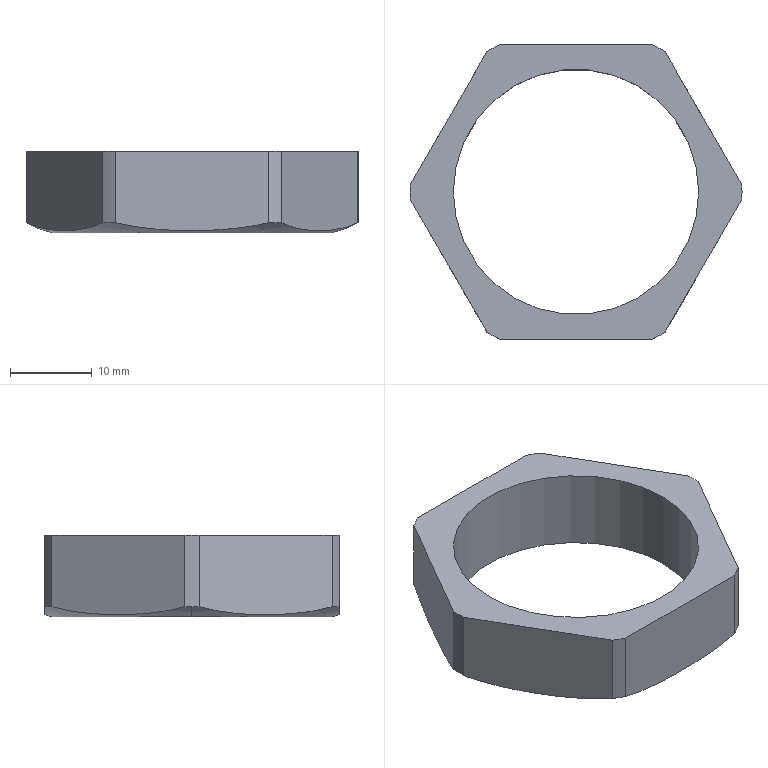Part | SolidWorks | features RefAxis 3, BaseBody 1 | 1 solid | 19 faces | box 40.6 x 36 x 10 mm | volume 4057 mm3 | cylinder 9 | plane 8 | spline 2 | commonest cylinder face diameters 40.6 x7 30 x2
STEP:
#1=CARTESIAN_POINT('',(35.75,19.99,0.));
#2=VERTEX_POINT('',#1);
#3=CARTESIAN_POINT('',(5.75,19.99,0.));
#4=VERTEX_POINT('',#3);
#5=CARTESIAN_POINT('',(20.75,19.99,0.));
#6=DIRECTION('',(0.,0.,-1.));
#7=DIRECTION('',(-1.,0.,0.));
#8=AXIS2_PLACEMENT_3D('',#5,#6,#7);
#9=CIRCLE('',#8,15.);
#10=EDGE_CURVE('',#2,#4,#9,.T.);
#11=ORIENTED_EDGE('',*,*,#10,.F.);
#12=CARTESIAN_POINT('',(35.75,19.99,-10.));
#13=VERTEX_POINT('',#12);
#14=CARTESIAN_POINT('',(35.75,19.99,0.));
#15=DIRECTION('',(0.,0.,-1.));
#16=VECTOR('',#15,1000.);
#17=LINE('',#14,#16);
#18=EDGE_CURVE('',#2,#13,#17,.T.);
#19=ORIENTED_EDGE('',*,*,#18,.T.);
#20=CARTESIAN_POINT('',(5.75,19.99,-10.));
#21=VERTEX_POINT('',#20);
#22=CARTESIAN_POINT('',(20.75,19.99,-10.));
#23=DIRECTION('',(0.,0.,1.));
#24=DIRECTION('',(-1.,0.,0.));
#25=AXIS2_PLACEMENT_3D('',#22,#23,#24);
#26=CIRCLE('',#25,15.);
#27=EDGE_CURVE('',#21,#13,#26,.T.);
#28=ORIENTED_EDGE('',*,*,#27,.F.);
#29=CARTESIAN_POINT('',(5.75,19.99,0.));
#30=DIRECTION('',(0.,0.,-1.));
#31=VECTOR('',#30,1000.);
#32=LINE('',#29,#31);
#33=EDGE_CURVE('',#4,#21,#32,.T.);
#34=ORIENTED_EDGE('',*,*,#33,.F.);
#35=EDGE_LOOP('',(#11,#19,#28,#34));
#36=FACE_OUTER_BOUND('',#35,.T.);
#37=CARTESIAN_POINT('',(20.75,19.99,0.));
#38=DIRECTION('',(0.,0.,-1.));
#39=DIRECTION('',(-1.,0.,0.));
#40=AXIS2_PLACEMENT_3D('',#37,#38,#39);
#41=CYLINDRICAL_SURFACE('',#40,15.);
#42=ADVANCED_FACE('',(#36),#41,.F.);
#43=CARTESIAN_POINT('',(41.031,19.118,-8.75));
#44=VERTEX_POINT('',#43);
#45=CARTESIAN_POINT('',(41.05,19.99,-8.75));
#46=VERTEX_POINT('',#45);
#47=CARTESIAN_POINT('',(20.75,19.99,-8.75));
#48=DIRECTION('',(0.,0.,1.));
#49=DIRECTION('',(1.,0.,0.));
#50=AXIS2_PLACEMENT_3D('',#47,#48,#49);
#51=CIRCLE('',#50,20.3);
#52=EDGE_CURVE('',#44,#46,#51,.T.);
#53=ORIENTED_EDGE('',*,*,#52,.T.);
#54=CARTESIAN_POINT('',(41.05,19.99,0.));
#55=VERTEX_POINT('',#54);
#56=CARTESIAN_POINT('',(41.05,19.99,-11.417));
#57=DIRECTION('',(0.,0.,1.));
#58=VECTOR('',#57,1000.);
#59=LINE('',#56,#58);
#60=EDGE_CURVE('',#46,#55,#59,.T.);
#61=ORIENTED_EDGE('',*,*,#60,.T.);
#62=CARTESIAN_POINT('',(41.031,19.118,0.));
#63=VERTEX_POINT('',#62);
#64=CARTESIAN_POINT('',(20.75,19.99,0.));
#65=DIRECTION('',(0.,0.,-1.));
#66=DIRECTION('',(1.,0.,0.));
#67=AXIS2_PLACEMENT_3D('',#64,#65,#66);
#68=CIRCLE('',#67,20.3);
#69=EDGE_CURVE('',#55,#63,#68,.T.);
#70=ORIENTED_EDGE('',*,*,#69,.T.);
#71=CARTESIAN_POINT('',(41.031,19.118,0.));
#72=DIRECTION('',(0.,0.,-1.));
#73=VECTOR('',#72,1000.);
#74=LINE('',#71,#73);
#75=EDGE_CURVE('',#63,#44,#74,.T.);
#76=ORIENTED_EDGE('',*,*,#75,.T.);
#77=EDGE_LOOP('',(#53,#61,#70,#76));
#78=FACE_OUTER_BOUND('',#77,.T.);
#79=CARTESIAN_POINT('',(20.75,19.99,-11.417));
#80=DIRECTION('',(0.,0.,1.));
#81=DIRECTION('',(1.,0.,0.));
#82=AXIS2_PLACEMENT_3D('',#79,#80,#81);
#83=CYLINDRICAL_SURFACE('',#82,20.3);
#84=ADVANCED_FACE('',(#78),#83,.T.);
#85=ORIENTED_EDGE('',*,*,#18,.F.);
#86=CARTESIAN_POINT('',(20.75,19.99,0.));
#87=DIRECTION('',(0.,0.,-1.));
#88=DIRECTION('',(-1.,0.,0.));
#89=AXIS2_PLACEMENT_3D('',#86,#87,#88);
#90=CIRCLE('',#89,15.);
#91=EDGE_CURVE('',#4,#2,#90,.T.);
#92=ORIENTED_EDGE('',*,*,#91,.F.);
#93=ORIENTED_EDGE('',*,*,#33,.T.);
#94=CARTESIAN_POINT('',(20.75,19.99,-10.));
#95=DIRECTION('',(0.,0.,1.));
#96=DIRECTION('',(-1.,0.,0.));
#97=AXIS2_PLACEMENT_3D('',#94,#95,#96);
#98=CIRCLE('',#97,15.);
#99=EDGE_CURVE('',#13,#21,#98,.T.);
#100=ORIENTED_EDGE('',*,*,#99,.F.);
#101=EDGE_LOOP('',(#85,#92,#93,#100));
#102=FACE_OUTER_BOUND('',#101,.T.);
#103=CARTESIAN_POINT('',(20.75,19.99,0.));
#104=DIRECTION('',(0.,0.,-1.));
#105=DIRECTION('',(-1.,0.,0.));
#106=AXIS2_PLACEMENT_3D('',#103,#104,#105);
#107=CYLINDRICAL_SURFACE('',#106,15.);
#108=ADVANCED_FACE('',(#102),#107,.F.);
#109=ORIENTED_EDGE('',*,*,#91,.T.);
#110=ORIENTED_EDGE('',*,*,#10,.T.);
#111=EDGE_LOOP('',(#109,#110));
#112=FACE_BOUND('',#111,.T.);
#113=CARTESIAN_POINT('',(41.031,20.862,0.));
#114=VERTEX_POINT('',#113);
#115=CARTESIAN_POINT('',(20.75,19.99,0.));
#116=DIRECTION('',(0.,0.,-1.));
#117=DIRECTION('',(1.,0.,0.));
#118=AXIS2_PLACEMENT_3D('',#115,#116,#117);
#119=CIRCLE('',#118,20.3);
#120=EDGE_CURVE('',#114,#55,#119,.T.);
#121=ORIENTED_EDGE('',*,*,#120,.F.);
#122=CARTESIAN_POINT('',(31.646,37.118,0.));
#123=VERTEX_POINT('',#122);
#124=CARTESIAN_POINT('',(41.031,20.862,0.));
#125=DIRECTION('',(-0.5,0.866,0.));
#126=VECTOR('',#125,1000.);
#127=LINE('',#124,#126);
#128=EDGE_CURVE('',#114,#123,#127,.T.);
#129=ORIENTED_EDGE('',*,*,#128,.T.);
#130=CARTESIAN_POINT('',(30.136,37.99,0.));
#131=VERTEX_POINT('',#130);
#132=CARTESIAN_POINT('',(20.75,19.99,0.));
#133=DIRECTION('',(0.,0.,1.));
#134=DIRECTION('',(1.,0.,0.));
#135=AXIS2_PLACEMENT_3D('',#132,#133,#134);
#136=CIRCLE('',#135,20.3);
#137=EDGE_CURVE('',#123,#131,#136,.T.);
#138=ORIENTED_EDGE('',*,*,#137,.T.);
#139=CARTESIAN_POINT('',(11.364,37.99,0.));
#140=VERTEX_POINT('',#139);
#141=CARTESIAN_POINT('',(41.535,37.99,0.));
#142=DIRECTION('',(-1.,0.,0.));
#143=VECTOR('',#142,1000.);
#144=LINE('',#141,#143);
#145=EDGE_CURVE('',#131,#140,#144,.T.);
#146=ORIENTED_EDGE('',*,*,#145,.T.);
#147=CARTESIAN_POINT('',(9.854,37.118,0.));
#148=VERTEX_POINT('',#147);
#149=CARTESIAN_POINT('',(20.75,19.99,0.));
#150=DIRECTION('',(0.,0.,1.));
#151=DIRECTION('',(1.,0.,0.));
#152=AXIS2_PLACEMENT_3D('',#149,#150,#151);
#153=CIRCLE('',#152,20.3);
#154=EDGE_CURVE('',#140,#148,#153,.T.);
#155=ORIENTED_EDGE('',*,*,#154,.T.);
#156=CARTESIAN_POINT('',(0.4687,20.862,0.));
#157=VERTEX_POINT('',#156);
#158=CARTESIAN_POINT('',(9.854,37.118,0.));
#159=DIRECTION('',(-0.5,-0.866,0.));
#160=VECTOR('',#159,1000.);
#161=LINE('',#158,#160);
#162=EDGE_CURVE('',#148,#157,#161,.T.);
#163=ORIENTED_EDGE('',*,*,#162,.T.);
#164=CARTESIAN_POINT('',(0.4687,19.118,0.));
#165=VERTEX_POINT('',#164);
#166=CARTESIAN_POINT('',(20.75,19.99,0.));
#167=DIRECTION('',(0.,0.,1.));
#168=DIRECTION('',(1.,0.,0.));
#169=AXIS2_PLACEMENT_3D('',#166,#167,#168);
#170=CIRCLE('',#169,20.3);
#171=EDGE_CURVE('',#157,#165,#170,.T.);
#172=ORIENTED_EDGE('',*,*,#171,.T.);
#173=CARTESIAN_POINT('',(9.854,2.862,0.));
#174=VERTEX_POINT('',#173);
#175=CARTESIAN_POINT('',(0.4687,19.118,0.));
#176=DIRECTION('',(0.5,-0.866,0.));
#177=VECTOR('',#176,1000.);
#178=LINE('',#175,#177);
#179=EDGE_CURVE('',#165,#174,#178,.T.);
#180=ORIENTED_EDGE('',*,*,#179,.T.);
#181=CARTESIAN_POINT('',(11.364,1.99,0.));
#182=VERTEX_POINT('',#181);
#183=CARTESIAN_POINT('',(20.75,19.99,0.));
#184=DIRECTION('',(0.,0.,1.));
#185=DIRECTION('',(1.,0.,0.));
#186=AXIS2_PLACEMENT_3D('',#183,#184,#185);
#187=CIRCLE('',#186,20.3);
#188=EDGE_CURVE('',#174,#182,#187,.T.);
#189=ORIENTED_EDGE('',*,*,#188,.T.);
#190=CARTESIAN_POINT('',(30.136,1.99,0.));
#191=VERTEX_POINT('',#190);
#192=CARTESIAN_POINT('',(41.535,1.99,0.));
#193=DIRECTION('',(1.,0.,0.));
#194=VECTOR('',#193,1000.);
#195=LINE('',#192,#194);
#196=EDGE_CURVE('',#182,#191,#195,.T.);
#197=ORIENTED_EDGE('',*,*,#196,.T.);
#198=CARTESIAN_POINT('',(31.646,2.862,0.));
#199=VERTEX_POINT('',#198);
#200=CARTESIAN_POINT('',(20.75,19.99,0.));
#201=DIRECTION('',(0.,0.,1.));
#202=DIRECTION('',(1.,0.,0.));
#203=AXIS2_PLACEMENT_3D('',#200,#201,#202);
#204=CIRCLE('',#203,20.3);
#205=EDGE_CURVE('',#191,#199,#204,.T.);
#206=ORIENTED_EDGE('',*,*,#205,.T.);
#207=CARTESIAN_POINT('',(31.646,2.862,0.));
#208=DIRECTION('',(0.5,0.866,0.));
#209=VECTOR('',#208,1000.);
#210=LINE('',#207,#209);
#211=EDGE_CURVE('',#199,#63,#210,.T.);
#212=ORIENTED_EDGE('',*,*,#211,.T.);
#213=ORIENTED_EDGE('',*,*,#69,.F.);
#214=EDGE_LOOP('',(#121,#129,#138,#146,#155,#163,#172,#180,#189,#197,#206,#212,#213));
#215=FACE_OUTER_BOUND('',#214,.T.);
#216=CARTESIAN_POINT('',(41.535,19.99,0.));
#217=DIRECTION('',(0.,0.,1.));
#218=DIRECTION('',(1.,0.,0.));
#219=AXIS2_PLACEMENT_3D('',#216,#217,#218);
#220=PLANE('',#219);
#221=ADVANCED_FACE('',(#112,#215),#220,.T.);
#222=ORIENTED_EDGE('',*,*,#27,.T.);
#223=ORIENTED_EDGE('',*,*,#99,.T.);
#224=EDGE_LOOP('',(#222,#223));
#225=FACE_BOUND('',#224,.T.);
#226=CARTESIAN_POINT('',(37.75,19.99,-10.));
#227=VERTEX_POINT('',#226);
#228=CARTESIAN_POINT('',(3.75,19.99,-10.));
#229=VERTEX_POINT('',#228);
#230=CARTESIAN_POINT('',(37.75,19.99,-10.));
#231=CARTESIAN_POINT('',(37.75,53.99,-10.));
#232=CARTESIAN_POINT('',(3.75,53.99,-10.));
#233=CARTESIAN_POINT('',(3.75,19.99,-10.));
#234=(BOUNDED_CURVE()B_SPLINE_CURVE(3,(#230,#231,#232,#233),.UNSPECIFIED.,.F.,.F.)B_SPLINE_CURVE_WITH_KNOTS((4,4),(0.,0.05314),.UNSPECIFIED.)CURVE()GEOMETRIC_REPRESENTATION_ITEM()RATIONAL_B_SPLINE_CURVE((1.,0.3333,0.3333,1.))REPRESENTATION_ITEM(''));
#235=EDGE_CURVE('',#227,#229,#234,.T.);
#236=ORIENTED_EDGE('',*,*,#235,.F.);
#237=CARTESIAN_POINT('',(3.75,19.99,-10.));
#238=CARTESIAN_POINT('',(3.75,-14.01,-10.));
#239=CARTESIAN_POINT('',(37.75,-14.01,-10.));
#240=CARTESIAN_POINT('',(37.75,19.99,-10.));
#241=(BOUNDED_CURVE()B_SPLINE_CURVE(3,(#237,#238,#239,#240),.UNSPECIFIED.,.F.,.F.)B_SPLINE_CURVE_WITH_KNOTS((4,4),(0.,0.05314),.UNSPECIFIED.)CURVE()GEOMETRIC_REPRESENTATION_ITEM()RATIONAL_B_SPLINE_CURVE((1.,0.3333,0.3333,1.))REPRESENTATION_ITEM(''));
#242=EDGE_CURVE('',#229,#227,#241,.T.);
#243=ORIENTED_EDGE('',*,*,#242,.F.);
#244=EDGE_LOOP('',(#236,#243));
#245=FACE_OUTER_BOUND('',#244,.T.);
#246=CARTESIAN_POINT('',(41.535,19.99,-10.));
#247=DIRECTION('',(0.,0.,1.));
#248=DIRECTION('',(1.,0.,0.));
#249=AXIS2_PLACEMENT_3D('',#246,#247,#248);
#250=PLANE('',#249);
#251=ADVANCED_FACE('',(#225,#245),#250,.F.);
#252=CARTESIAN_POINT('',(31.646,2.862,-8.75));
#253=VERTEX_POINT('',#252);
#254=CARTESIAN_POINT('',(31.646,2.862,0.));
#255=DIRECTION('',(0.,0.,1.));
#256=VECTOR('',#255,1000.);
#257=LINE('',#254,#256);
#258=EDGE_CURVE('',#253,#199,#257,.T.);
#259=ORIENTED_EDGE('',*,*,#258,.F.);
#260=CARTESIAN_POINT('',(41.031,19.118,-8.75));
#261=CARTESIAN_POINT('',(40.646,18.451,-8.942));
#262=CARTESIAN_POINT('',(40.258,17.778,-9.096));
#263=CARTESIAN_POINT('',(39.475,16.424,-9.345));
#264=CARTESIAN_POINT('',(39.081,15.74,-9.441));
#265=CARTESIAN_POINT('',(37.899,13.694,-9.662));
#266=CARTESIAN_POINT('',(37.114,12.333,-9.722));
#267=CARTESIAN_POINT('',(35.545,9.616,-9.721));
#268=CARTESIAN_POINT('',(34.762,8.259,-9.659));
#269=CARTESIAN_POINT('',(33.2,5.554,-9.367));
#270=CARTESIAN_POINT('',(32.421,4.205,-9.137));
#271=CARTESIAN_POINT('',(31.646,2.862,-8.75));
#272=B_SPLINE_CURVE_WITH_KNOTS('',3,(#260,#261,#262,#263,#264,#265,#266,#267,#268,#269,#270,#271),.UNSPECIFIED.,.F.,.F.,(4,2,2,2,2,4),(0.,0.002376,0.004751,0.009503,0.01425,0.01901),.UNSPECIFIED.);
#273=EDGE_CURVE('',#44,#253,#272,.T.);
#274=ORIENTED_EDGE('',*,*,#273,.F.);
#275=ORIENTED_EDGE('',*,*,#75,.F.);
#276=ORIENTED_EDGE('',*,*,#211,.F.);
#277=EDGE_LOOP('',(#259,#274,#275,#276));
#278=FACE_OUTER_BOUND('',#277,.T.);
#279=CARTESIAN_POINT('',(31.142,1.99,0.));
#280=DIRECTION('',(-0.866,0.5,0.));
#281=DIRECTION('',(-0.5,-0.866,0.));
#282=AXIS2_PLACEMENT_3D('',#279,#280,#281);
#283=PLANE('',#282);
#284=ADVANCED_FACE('',(#278),#283,.F.);
#285=ORIENTED_EDGE('',*,*,#205,.F.);
#286=CARTESIAN_POINT('',(30.136,1.99,-8.75));
#287=VERTEX_POINT('',#286);
#288=CARTESIAN_POINT('',(30.136,1.99,-11.417));
#289=DIRECTION('',(0.,0.,-1.));
#290=VECTOR('',#289,1000.);
#291=LINE('',#288,#290);
#292=EDGE_CURVE('',#191,#287,#291,.T.);
#293=ORIENTED_EDGE('',*,*,#292,.T.);
#294=CARTESIAN_POINT('',(20.75,19.99,-8.75));
#295=DIRECTION('',(0.,0.,1.));
#296=DIRECTION('',(1.,0.,0.));
#297=AXIS2_PLACEMENT_3D('',#294,#295,#296);
#298=CIRCLE('',#297,20.3);
#299=EDGE_CURVE('',#287,#253,#298,.T.);
#300=ORIENTED_EDGE('',*,*,#299,.T.);
#301=ORIENTED_EDGE('',*,*,#258,.T.);
#302=EDGE_LOOP('',(#285,#293,#300,#301));
#303=FACE_OUTER_BOUND('',#302,.T.);
#304=CARTESIAN_POINT('',(20.75,19.99,-11.417));
#305=DIRECTION('',(0.,0.,1.));
#306=DIRECTION('',(1.,0.,0.));
#307=AXIS2_PLACEMENT_3D('',#304,#305,#306);
#308=CYLINDRICAL_SURFACE('',#307,20.3);
#309=ADVANCED_FACE('',(#303),#308,.T.);
#310=CARTESIAN_POINT('',(11.364,1.99,-8.75));
#311=VERTEX_POINT('',#310);
#312=CARTESIAN_POINT('',(11.364,1.99,0.));
#313=DIRECTION('',(0.,0.,1.));
#314=VECTOR('',#313,1000.);
#315=LINE('',#312,#314);
#316=EDGE_CURVE('',#311,#182,#315,.T.);
#317=ORIENTED_EDGE('',*,*,#316,.F.);
#318=CARTESIAN_POINT('',(30.136,1.99,-8.75));
#319=CARTESIAN_POINT('',(28.596,1.99,-9.134));
#320=CARTESIAN_POINT('',(27.029,1.99,-9.367));
#321=CARTESIAN_POINT('',(23.875,1.99,-9.662));
#322=CARTESIAN_POINT('',(22.302,1.99,-9.722));
#323=CARTESIAN_POINT('',(19.162,1.99,-9.721));
#324=CARTESIAN_POINT('',(17.596,1.99,-9.659));
#325=CARTESIAN_POINT('',(14.472,1.99,-9.367));
#326=CARTESIAN_POINT('',(12.914,1.99,-9.136));
#327=CARTESIAN_POINT('',(11.364,1.99,-8.75));
#328=B_SPLINE_CURVE_WITH_KNOTS('',3,(#318,#319,#320,#321,#322,#323,#324,#325,#326,#327),.UNSPECIFIED.,.F.,.F.,(4,2,2,2,4),(0.,0.004746,0.009492,0.01424,0.01898),.UNSPECIFIED.);
#329=EDGE_CURVE('',#287,#311,#328,.T.);
#330=ORIENTED_EDGE('',*,*,#329,.F.);
#331=ORIENTED_EDGE('',*,*,#292,.F.);
#332=ORIENTED_EDGE('',*,*,#196,.F.);
#333=EDGE_LOOP('',(#317,#330,#331,#332));
#334=FACE_OUTER_BOUND('',#333,.T.);
#335=CARTESIAN_POINT('',(10.358,1.99,0.));
#336=DIRECTION('',(0.,1.,0.));
#337=DIRECTION('',(-1.,0.,0.));
#338=AXIS2_PLACEMENT_3D('',#335,#336,#337);
#339=PLANE('',#338);
#340=ADVANCED_FACE('',(#334),#339,.F.);
#341=ORIENTED_EDGE('',*,*,#188,.F.);
#342=CARTESIAN_POINT('',(9.854,2.862,-8.75));
#343=VERTEX_POINT('',#342);
#344=CARTESIAN_POINT('',(9.854,2.862,-11.417));
#345=DIRECTION('',(0.,0.,-1.));
#346=VECTOR('',#345,1000.);
#347=LINE('',#344,#346);
#348=EDGE_CURVE('',#174,#343,#347,.T.);
#349=ORIENTED_EDGE('',*,*,#348,.T.);
#350=CARTESIAN_POINT('',(20.75,19.99,-8.75));
#351=DIRECTION('',(0.,0.,1.));
#352=DIRECTION('',(1.,0.,0.));
#353=AXIS2_PLACEMENT_3D('',#350,#351,#352);
#354=CIRCLE('',#353,20.3);
#355=EDGE_CURVE('',#343,#311,#354,.T.);
#356=ORIENTED_EDGE('',*,*,#355,.T.);
#357=ORIENTED_EDGE('',*,*,#316,.T.);
#358=EDGE_LOOP('',(#341,#349,#356,#357));
#359=FACE_OUTER_BOUND('',#358,.T.);
#360=CARTESIAN_POINT('',(20.75,19.99,-11.417));
#361=DIRECTION('',(0.,0.,1.));
#362=DIRECTION('',(1.,0.,0.));
#363=AXIS2_PLACEMENT_3D('',#360,#361,#362);
#364=CYLINDRICAL_SURFACE('',#363,20.3);
#365=ADVANCED_FACE('',(#359),#364,.T.);
#366=CARTESIAN_POINT('',(0.4687,19.118,-8.75));
#367=VERTEX_POINT('',#366);
#368=CARTESIAN_POINT('',(0.4687,19.118,0.));
#369=DIRECTION('',(0.,0.,1.));
#370=VECTOR('',#369,1000.);
#371=LINE('',#368,#370);
#372=EDGE_CURVE('',#367,#165,#371,.T.);
#373=ORIENTED_EDGE('',*,*,#372,.F.);
#374=CARTESIAN_POINT('',(9.854,2.862,-8.75));
#375=CARTESIAN_POINT('',(9.084,4.195,-9.134));
#376=CARTESIAN_POINT('',(8.301,5.552,-9.367));
#377=CARTESIAN_POINT('',(6.724,8.284,-9.662));
#378=CARTESIAN_POINT('',(5.937,9.646,-9.722));
#379=CARTESIAN_POINT('',(4.368,12.365,-9.721));
#380=CARTESIAN_POINT('',(3.584,13.722,-9.659));
#381=CARTESIAN_POINT('',(2.022,16.427,-9.367));
#382=CARTESIAN_POINT('',(1.244,17.776,-9.136));
#383=CARTESIAN_POINT('',(0.4687,19.118,-8.75));
#384=B_SPLINE_CURVE_WITH_KNOTS('',3,(#374,#375,#376,#377,#378,#379,#380,#381,#382,#383),.UNSPECIFIED.,.F.,.F.,(4,2,2,2,4),(0.,0.004746,0.009492,0.01424,0.01898),.UNSPECIFIED.);
#385=EDGE_CURVE('',#343,#367,#384,.T.);
#386=ORIENTED_EDGE('',*,*,#385,.F.);
#387=ORIENTED_EDGE('',*,*,#348,.F.);
#388=ORIENTED_EDGE('',*,*,#179,.F.);
#389=EDGE_LOOP('',(#373,#386,#387,#388));
#390=FACE_OUTER_BOUND('',#389,.T.);
#391=CARTESIAN_POINT('',(-0.03461,19.99,0.));
#392=DIRECTION('',(0.866,0.5,0.));
#393=DIRECTION('',(-0.5,0.866,0.));
#394=AXIS2_PLACEMENT_3D('',#391,#392,#393);
#395=PLANE('',#394);
#396=ADVANCED_FACE('',(#390),#395,.F.);
#397=CARTESIAN_POINT('',(0.4687,20.862,-8.75));
#398=VERTEX_POINT('',#397);
#399=CARTESIAN_POINT('',(0.4687,20.862,-11.417));
#400=DIRECTION('',(0.,0.,-1.));
#401=VECTOR('',#400,1000.);
#402=LINE('',#399,#401);
#403=EDGE_CURVE('',#157,#398,#402,.T.);
#404=ORIENTED_EDGE('',*,*,#403,.T.);
#405=CARTESIAN_POINT('',(0.45,19.99,-8.75));
#406=VERTEX_POINT('',#405);
#407=CARTESIAN_POINT('',(20.75,19.99,-8.75));
#408=DIRECTION('',(0.,0.,1.));
#409=DIRECTION('',(1.,0.,0.));
#410=AXIS2_PLACEMENT_3D('',#407,#408,#409);
#411=CIRCLE('',#410,20.3);
#412=EDGE_CURVE('',#398,#406,#411,.T.);
#413=ORIENTED_EDGE('',*,*,#412,.T.);
#414=CARTESIAN_POINT('',(20.75,19.99,-8.75));
#415=DIRECTION('',(0.,0.,1.));
#416=DIRECTION('',(1.,0.,0.));
#417=AXIS2_PLACEMENT_3D('',#414,#415,#416);
#418=CIRCLE('',#417,20.3);
#419=EDGE_CURVE('',#406,#367,#418,.T.);
#420=ORIENTED_EDGE('',*,*,#419,.T.);
#421=ORIENTED_EDGE('',*,*,#372,.T.);
#422=ORIENTED_EDGE('',*,*,#171,.F.);
#423=EDGE_LOOP('',(#404,#413,#420,#421,#422));
#424=FACE_OUTER_BOUND('',#423,.T.);
#425=CARTESIAN_POINT('',(20.75,19.99,-11.417));
#426=DIRECTION('',(0.,0.,1.));
#427=DIRECTION('',(1.,0.,0.));
#428=AXIS2_PLACEMENT_3D('',#425,#426,#427);
#429=CYLINDRICAL_SURFACE('',#428,20.3);
#430=ADVANCED_FACE('',(#424),#429,.T.);
#431=CARTESIAN_POINT('',(9.854,37.118,-8.75));
#432=VERTEX_POINT('',#431);
#433=CARTESIAN_POINT('',(9.854,37.118,0.));
#434=DIRECTION('',(0.,0.,1.));
#435=VECTOR('',#434,1000.);
#436=LINE('',#433,#435);
#437=EDGE_CURVE('',#432,#148,#436,.T.);
#438=ORIENTED_EDGE('',*,*,#437,.F.);
#439=CARTESIAN_POINT('',(0.4687,20.862,-8.75));
#440=CARTESIAN_POINT('',(0.8539,21.529,-8.942));
#441=CARTESIAN_POINT('',(1.242,22.202,-9.096));
#442=CARTESIAN_POINT('',(2.025,23.556,-9.345));
#443=CARTESIAN_POINT('',(2.419,24.24,-9.441));
#444=CARTESIAN_POINT('',(3.601,26.286,-9.662));
#445=CARTESIAN_POINT('',(4.386,27.647,-9.722));
#446=CARTESIAN_POINT('',(5.955,30.364,-9.721));
#447=CARTESIAN_POINT('',(6.738,31.721,-9.659));
#448=CARTESIAN_POINT('',(8.3,34.426,-9.367));
#449=CARTESIAN_POINT('',(9.079,35.775,-9.137));
#450=CARTESIAN_POINT('',(9.854,37.118,-8.75));
#451=B_SPLINE_CURVE_WITH_KNOTS('',3,(#439,#440,#441,#442,#443,#444,#445,#446,#447,#448,#449,#450),.UNSPECIFIED.,.F.,.F.,(4,2,2,2,2,4),(0.,0.002376,0.004751,0.009503,0.01425,0.01901),.UNSPECIFIED.);
#452=EDGE_CURVE('',#398,#432,#451,.T.);
#453=ORIENTED_EDGE('',*,*,#452,.F.);
#454=ORIENTED_EDGE('',*,*,#403,.F.);
#455=ORIENTED_EDGE('',*,*,#162,.F.);
#456=EDGE_LOOP('',(#438,#453,#454,#455));
#457=FACE_OUTER_BOUND('',#456,.T.);
#458=CARTESIAN_POINT('',(10.358,37.99,0.));
#459=DIRECTION('',(0.866,-0.5,0.));
#460=DIRECTION('',(0.5,0.866,0.));
#461=AXIS2_PLACEMENT_3D('',#458,#459,#460);
#462=PLANE('',#461);
#463=ADVANCED_FACE('',(#457),#462,.F.);
#464=ORIENTED_EDGE('',*,*,#154,.F.);
#465=CARTESIAN_POINT('',(11.364,37.99,-8.75));
#466=VERTEX_POINT('',#465);
#467=CARTESIAN_POINT('',(11.364,37.99,-11.417));
#468=DIRECTION('',(0.,0.,-1.));
#469=VECTOR('',#468,1000.);
#470=LINE('',#467,#469);
#471=EDGE_CURVE('',#140,#466,#470,.T.);
#472=ORIENTED_EDGE('',*,*,#471,.T.);
#473=CARTESIAN_POINT('',(20.75,19.99,-8.75));
#474=DIRECTION('',(0.,0.,1.));
#475=DIRECTION('',(1.,0.,0.));
#476=AXIS2_PLACEMENT_3D('',#473,#474,#475);
#477=CIRCLE('',#476,20.3);
#478=EDGE_CURVE('',#466,#432,#477,.T.);
#479=ORIENTED_EDGE('',*,*,#478,.T.);
#480=ORIENTED_EDGE('',*,*,#437,.T.);
#481=EDGE_LOOP('',(#464,#472,#479,#480));
#482=FACE_OUTER_BOUND('',#481,.T.);
#483=CARTESIAN_POINT('',(20.75,19.99,-11.417));
#484=DIRECTION('',(0.,0.,1.));
#485=DIRECTION('',(1.,0.,0.));
#486=AXIS2_PLACEMENT_3D('',#483,#484,#485);
#487=CYLINDRICAL_SURFACE('',#486,20.3);
#488=ADVANCED_FACE('',(#482),#487,.T.);
#489=CARTESIAN_POINT('',(30.136,37.99,-8.75));
#490=VERTEX_POINT('',#489);
#491=CARTESIAN_POINT('',(30.136,37.99,0.));
#492=DIRECTION('',(0.,0.,1.));
#493=VECTOR('',#492,1000.);
#494=LINE('',#491,#493);
#495=EDGE_CURVE('',#490,#131,#494,.T.);
#496=ORIENTED_EDGE('',*,*,#495,.F.);
#497=CARTESIAN_POINT('',(11.364,37.99,-8.75));
#498=CARTESIAN_POINT('',(12.904,37.99,-9.134));
#499=CARTESIAN_POINT('',(14.471,37.99,-9.367));
#500=CARTESIAN_POINT('',(17.625,37.99,-9.662));
#501=CARTESIAN_POINT('',(19.198,37.99,-9.722));
#502=CARTESIAN_POINT('',(22.338,37.99,-9.721));
#503=CARTESIAN_POINT('',(23.904,37.99,-9.659));
#504=CARTESIAN_POINT('',(27.028,37.99,-9.367));
#505=CARTESIAN_POINT('',(28.586,37.99,-9.136));
#506=CARTESIAN_POINT('',(30.136,37.99,-8.75));
#507=B_SPLINE_CURVE_WITH_KNOTS('',3,(#497,#498,#499,#500,#501,#502,#503,#504,#505,#506),.UNSPECIFIED.,.F.,.F.,(4,2,2,2,4),(0.,0.004746,0.009492,0.01424,0.01898),.UNSPECIFIED.);
#508=EDGE_CURVE('',#466,#490,#507,.T.);
#509=ORIENTED_EDGE('',*,*,#508,.F.);
#510=ORIENTED_EDGE('',*,*,#471,.F.);
#511=ORIENTED_EDGE('',*,*,#145,.F.);
#512=EDGE_LOOP('',(#496,#509,#510,#511));
#513=FACE_OUTER_BOUND('',#512,.T.);
#514=CARTESIAN_POINT('',(31.142,37.99,0.));
#515=DIRECTION('',(0.,-1.,0.));
#516=DIRECTION('',(1.,0.,0.));
#517=AXIS2_PLACEMENT_3D('',#514,#515,#516);
#518=PLANE('',#517);
#519=ADVANCED_FACE('',(#513),#518,.F.);
#520=ORIENTED_EDGE('',*,*,#137,.F.);
#521=CARTESIAN_POINT('',(31.646,37.118,-8.75));
#522=VERTEX_POINT('',#521);
#523=CARTESIAN_POINT('',(31.646,37.118,-11.417));
#524=DIRECTION('',(0.,0.,-1.));
#525=VECTOR('',#524,1000.);
#526=LINE('',#523,#525);
#527=EDGE_CURVE('',#123,#522,#526,.T.);
#528=ORIENTED_EDGE('',*,*,#527,.T.);
#529=CARTESIAN_POINT('',(20.75,19.99,-8.75));
#530=DIRECTION('',(0.,0.,1.));
#531=DIRECTION('',(1.,0.,0.));
#532=AXIS2_PLACEMENT_3D('',#529,#530,#531);
#533=CIRCLE('',#532,20.3);
#534=EDGE_CURVE('',#522,#490,#533,.T.);
#535=ORIENTED_EDGE('',*,*,#534,.T.);
#536=ORIENTED_EDGE('',*,*,#495,.T.);
#537=EDGE_LOOP('',(#520,#528,#535,#536));
#538=FACE_OUTER_BOUND('',#537,.T.);
#539=CARTESIAN_POINT('',(20.75,19.99,-11.417));
#540=DIRECTION('',(0.,0.,1.));
#541=DIRECTION('',(1.,0.,0.));
#542=AXIS2_PLACEMENT_3D('',#539,#540,#541);
#543=CYLINDRICAL_SURFACE('',#542,20.3);
#544=ADVANCED_FACE('',(#538),#543,.T.);
#545=CARTESIAN_POINT('',(41.031,20.862,-8.75));
#546=VERTEX_POINT('',#545);
#547=CARTESIAN_POINT('',(41.031,20.862,0.));
#548=DIRECTION('',(0.,0.,1.));
#549=VECTOR('',#548,1000.);
#550=LINE('',#547,#549);
#551=EDGE_CURVE('',#546,#114,#550,.T.);
#552=ORIENTED_EDGE('',*,*,#551,.F.);
#553=CARTESIAN_POINT('',(31.646,37.118,-8.75));
#554=CARTESIAN_POINT('',(32.416,35.785,-9.134));
#555=CARTESIAN_POINT('',(33.199,34.428,-9.367));
#556=CARTESIAN_POINT('',(34.776,31.696,-9.662));
#557=CARTESIAN_POINT('',(35.563,30.334,-9.722));
#558=CARTESIAN_POINT('',(37.132,27.615,-9.721));
#559=CARTESIAN_POINT('',(37.916,26.258,-9.659));
#560=CARTESIAN_POINT('',(39.478,23.553,-9.367));
#561=CARTESIAN_POINT('',(40.256,22.204,-9.136));
#562=CARTESIAN_POINT('',(41.031,20.862,-8.75));
#563=B_SPLINE_CURVE_WITH_KNOTS('',3,(#553,#554,#555,#556,#557,#558,#559,#560,#561,#562),.UNSPECIFIED.,.F.,.F.,(4,2,2,2,4),(0.,0.004746,0.009492,0.01424,0.01898),.UNSPECIFIED.);
#564=EDGE_CURVE('',#522,#546,#563,.T.);
#565=ORIENTED_EDGE('',*,*,#564,.F.);
#566=ORIENTED_EDGE('',*,*,#527,.F.);
#567=ORIENTED_EDGE('',*,*,#128,.F.);
#568=EDGE_LOOP('',(#552,#565,#566,#567));
#569=FACE_OUTER_BOUND('',#568,.T.);
#570=CARTESIAN_POINT('',(41.535,19.99,0.));
#571=DIRECTION('',(-0.866,-0.5,0.));
#572=DIRECTION('',(0.5,-0.866,0.));
#573=AXIS2_PLACEMENT_3D('',#570,#571,#572);
#574=PLANE('',#573);
#575=ADVANCED_FACE('',(#569),#574,.F.);
#576=CARTESIAN_POINT('',(41.05,19.99,-8.75));
#577=CARTESIAN_POINT('',(39.526,19.99,-9.572));
#578=CARTESIAN_POINT('',(37.75,19.99,-10.));
#579=B_SPLINE_CURVE_WITH_KNOTS('',2,(#576,#577,#578),.UNSPECIFIED.,.F.,.F.,(3,3),(0.,0.5466),.UNSPECIFIED.);
#580=EDGE_CURVE('',#46,#227,#579,.T.);
#581=ORIENTED_EDGE('',*,*,#580,.F.);
#582=ORIENTED_EDGE('',*,*,#52,.F.);
#583=ORIENTED_EDGE('',*,*,#273,.T.);
#584=ORIENTED_EDGE('',*,*,#299,.F.);
#585=ORIENTED_EDGE('',*,*,#329,.T.);
#586=ORIENTED_EDGE('',*,*,#355,.F.);
#587=ORIENTED_EDGE('',*,*,#385,.T.);
#588=ORIENTED_EDGE('',*,*,#419,.F.);
#589=CARTESIAN_POINT('',(3.75,19.99,-10.));
#590=CARTESIAN_POINT('',(1.974,19.99,-9.572));
#591=CARTESIAN_POINT('',(0.45,19.99,-8.75));
#592=B_SPLINE_CURVE_WITH_KNOTS('',2,(#589,#590,#591),.UNSPECIFIED.,.F.,.F.,(3,3),(0.,0.5466),.UNSPECIFIED.);
#593=EDGE_CURVE('',#229,#406,#592,.T.);
#594=ORIENTED_EDGE('',*,*,#593,.F.);
#595=ORIENTED_EDGE('',*,*,#242,.T.);
#596=EDGE_LOOP('',(#581,#582,#583,#584,#585,#586,#587,#588,#594,#595));
#597=FACE_OUTER_BOUND('',#596,.T.);
#598=CARTESIAN_POINT('',(4.206,19.99,-10.11));
#599=CARTESIAN_POINT('',(4.206,-13.098,-10.11));
#600=CARTESIAN_POINT('',(37.294,-13.098,-10.11));
#601=CARTESIAN_POINT('',(37.294,19.99,-10.11));
#602=CARTESIAN_POINT('',(3.978,19.99,-10.055));
#603=CARTESIAN_POINT('',(3.978,-13.554,-10.055));
#604=CARTESIAN_POINT('',(37.522,-13.554,-10.055));
#605=CARTESIAN_POINT('',(37.522,19.99,-10.055));
#606=CARTESIAN_POINT('',(3.75,19.99,-10.));
#607=CARTESIAN_POINT('',(3.75,-14.01,-10.));
#608=CARTESIAN_POINT('',(37.75,-14.01,-10.));
#609=CARTESIAN_POINT('',(37.75,19.99,-10.));
#610=CARTESIAN_POINT('',(1.974,19.99,-9.572));
#611=CARTESIAN_POINT('',(1.974,-17.562,-9.572));
#612=CARTESIAN_POINT('',(39.526,-17.562,-9.572));
#613=CARTESIAN_POINT('',(39.526,19.99,-9.572));
#614=CARTESIAN_POINT('',(0.45,19.99,-8.75));
#615=CARTESIAN_POINT('',(0.45,-20.61,-8.75));
#616=CARTESIAN_POINT('',(41.05,-20.61,-8.75));
#617=CARTESIAN_POINT('',(41.05,19.99,-8.75));
#618=(BOUNDED_SURFACE()B_SPLINE_SURFACE(2,3,((#598,#599,#600,#601),(#602,#603,#604,#605),(#606,#607,#608,#609),(#610,#611,#612,#613),(#614,#615,#616,#617)),.UNSPECIFIED.,.F.,.F.,.F.)B_SPLINE_SURFACE_WITH_KNOTS((3,2,3),(4,4),(-0.07018,0.,0.5466),(0.,1.),.UNSPECIFIED.)GEOMETRIC_REPRESENTATION_ITEM()RATIONAL_B_SPLINE_SURFACE(((1.,0.3333,0.3333,1.),(1.,0.3333,0.3333,1.),(1.,0.3333,0.3333,1.),(1.,0.3333,0.3333,1.),(1.,0.3333,0.3333,1.)))REPRESENTATION_ITEM('')SURFACE());
#619=ADVANCED_FACE('',(#597),#618,.F.);
#620=ORIENTED_EDGE('',*,*,#235,.T.);
#621=ORIENTED_EDGE('',*,*,#593,.T.);
#622=ORIENTED_EDGE('',*,*,#412,.F.);
#623=ORIENTED_EDGE('',*,*,#452,.T.);
#624=ORIENTED_EDGE('',*,*,#478,.F.);
#625=ORIENTED_EDGE('',*,*,#508,.T.);
#626=ORIENTED_EDGE('',*,*,#534,.F.);
#627=ORIENTED_EDGE('',*,*,#564,.T.);
#628=CARTESIAN_POINT('',(20.75,19.99,-8.75));
#629=DIRECTION('',(0.,0.,1.));
#630=DIRECTION('',(0.,-1.,0.));
#631=AXIS2_PLACEMENT_3D('',#628,#629,#630);
#632=CIRCLE('',#631,20.3);
#633=EDGE_CURVE('',#46,#546,#632,.T.);
#634=ORIENTED_EDGE('',*,*,#633,.F.);
#635=ORIENTED_EDGE('',*,*,#580,.T.);
#636=EDGE_LOOP('',(#620,#621,#622,#623,#624,#625,#626,#627,#634,#635));
#637=FACE_OUTER_BOUND('',#636,.T.);
#638=CARTESIAN_POINT('',(37.294,19.99,-10.11));
#639=CARTESIAN_POINT('',(37.294,53.078,-10.11));
#640=CARTESIAN_POINT('',(4.206,53.078,-10.11));
#641=CARTESIAN_POINT('',(4.206,19.99,-10.11));
#642=CARTESIAN_POINT('',(37.522,19.99,-10.055));
#643=CARTESIAN_POINT('',(37.522,53.534,-10.055));
#644=CARTESIAN_POINT('',(3.978,53.534,-10.055));
#645=CARTESIAN_POINT('',(3.978,19.99,-10.055));
#646=CARTESIAN_POINT('',(37.75,19.99,-10.));
#647=CARTESIAN_POINT('',(37.75,53.99,-10.));
#648=CARTESIAN_POINT('',(3.75,53.99,-10.));
#649=CARTESIAN_POINT('',(3.75,19.99,-10.));
#650=CARTESIAN_POINT('',(39.526,19.99,-9.572));
#651=CARTESIAN_POINT('',(39.526,57.542,-9.572));
#652=CARTESIAN_POINT('',(1.974,57.542,-9.572));
#653=CARTESIAN_POINT('',(1.974,19.99,-9.572));
#654=CARTESIAN_POINT('',(41.05,19.99,-8.75));
#655=CARTESIAN_POINT('',(41.05,60.59,-8.75));
#656=CARTESIAN_POINT('',(0.45,60.59,-8.75));
#657=CARTESIAN_POINT('',(0.45,19.99,-8.75));
#658=(BOUNDED_SURFACE()B_SPLINE_SURFACE(2,3,((#638,#639,#640,#641),(#642,#643,#644,#645),(#646,#647,#648,#649),(#650,#651,#652,#653),(#654,#655,#656,#657)),.UNSPECIFIED.,.F.,.F.,.T.)B_SPLINE_SURFACE_WITH_KNOTS((3,2,3),(4,4),(-0.07018,0.,0.5466),(0.,1.),.UNSPECIFIED.)GEOMETRIC_REPRESENTATION_ITEM()RATIONAL_B_SPLINE_SURFACE(((1.,0.3333,0.3333,1.),(1.,0.3333,0.3333,1.),(1.,0.3333,0.3333,1.),(1.,0.3333,0.3333,1.),(1.,0.3333,0.3333,1.)))REPRESENTATION_ITEM('')SURFACE());
#659=ADVANCED_FACE('',(#637),#658,.F.);
#660=ORIENTED_EDGE('',*,*,#60,.F.);
#661=ORIENTED_EDGE('',*,*,#633,.T.);
#662=ORIENTED_EDGE('',*,*,#551,.T.);
#663=ORIENTED_EDGE('',*,*,#120,.T.);
#664=EDGE_LOOP('',(#660,#661,#662,#663));
#665=FACE_OUTER_BOUND('',#664,.T.);
#666=CARTESIAN_POINT('',(20.75,19.99,-11.417));
#667=DIRECTION('',(0.,0.,1.));
#668=DIRECTION('',(1.,0.,0.));
#669=AXIS2_PLACEMENT_3D('',#666,#667,#668);
#670=CYLINDRICAL_SURFACE('',#669,20.3);
#671=ADVANCED_FACE('',(#665),#670,.T.);
#672=CLOSED_SHELL('',(#42,#84,#108,#221,#251,#284,#309,#340,#365,#396,#430,#463,#488,#519,#544,#575,#619,#659,#671));
#673=MANIFOLD_SOLID_BREP('',#672);
#674=CARTESIAN_POINT('',(0.,0.,0.));
#675=DIRECTION('',(0.,0.,1.));
#676=DIRECTION('',(1.,0.,0.));
#677=AXIS2_PLACEMENT_3D('',#674,#675,#676);
#678=(LENGTH_UNIT()NAMED_UNIT(*)SI_UNIT(.MILLI.,.METRE.));
#679=UNCERTAINTY_MEASURE_WITH_UNIT(LENGTH_MEASURE(0.00001),#678,'','');
#680=(NAMED_UNIT(*)PLANE_ANGLE_UNIT()SI_UNIT($,.RADIAN.));
#681=(NAMED_UNIT(*)SI_UNIT($,.STERADIAN.)SOLID_ANGLE_UNIT());
#682=(GEOMETRIC_REPRESENTATION_CONTEXT(3)GLOBAL_UNCERTAINTY_ASSIGNED_CONTEXT((#679))GLOBAL_UNIT_ASSIGNED_CONTEXT((#678,#680,#681))REPRESENTATION_CONTEXT('',''));
#683=ADVANCED_BREP_SHAPE_REPRESENTATION('',(#673,#677),#682);